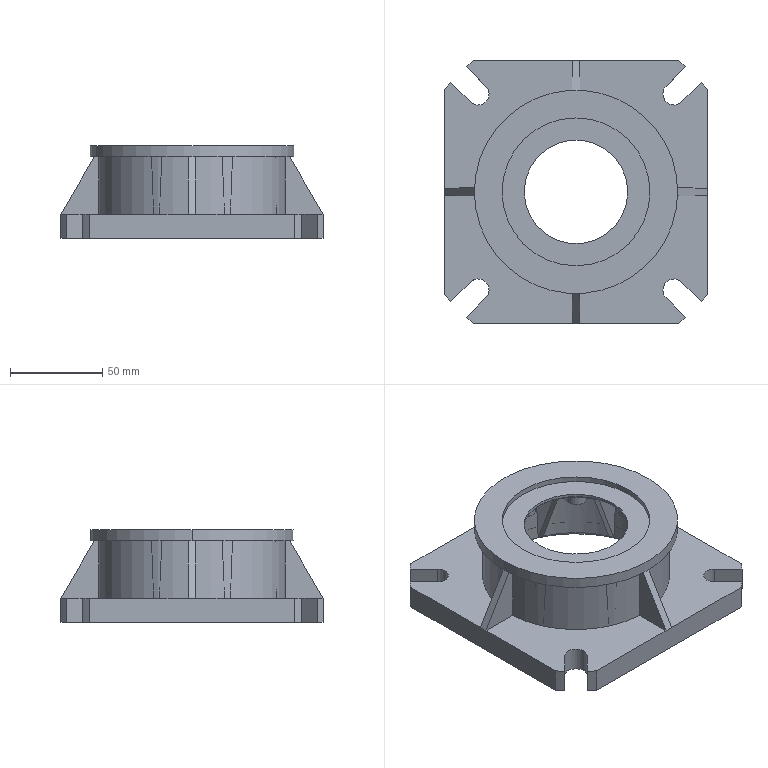Part | STEP file | Output flange_063_ZB.step_1 | 1 solid | 483 faces | box 142 x 142 x 50 mm | volume 173016 mm3 | plane 401 | cylinder 80 | cone 2 | commonest cylinder face diameters 126.5 x21 11.012 x16 100.05 x9 168.5 x8 180 x8 12 x6